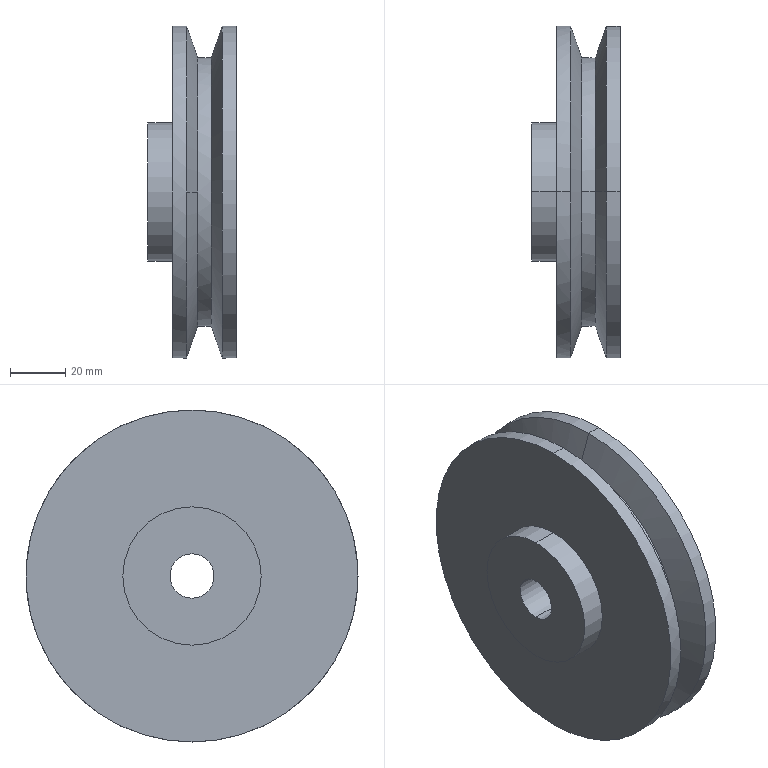Part | SolidWorks | features BaseBody 1 | 1 solid | 17 faces | box 32 x 120 x 120 mm | volume 235868 mm3 | cylinder 10 | cone 4 | plane 3 | commonest cylinder face diameters 120 x4 16 x2 50 x2 97.1 x2
STEP:
#1=CARTESIAN_POINT('',(-11.,0.,8.));
#2=VERTEX_POINT('',#1);
#3=CARTESIAN_POINT('',(-11.,0.,-8.));
#4=VERTEX_POINT('',#3);
#5=CARTESIAN_POINT('',(-11.,0.,0.));
#6=DIRECTION('',(1.,0.,0.));
#7=DIRECTION('',(0.,0.,-1.));
#8=AXIS2_PLACEMENT_3D('',#5,#6,#7);
#9=CIRCLE('',#8,8.);
#10=EDGE_CURVE('',#2,#4,#9,.T.);
#11=ORIENTED_EDGE('',*,*,#10,.F.);
#12=CARTESIAN_POINT('',(21.,0.,8.));
#13=VERTEX_POINT('',#12);
#14=CARTESIAN_POINT('',(0.,0.,8.));
#15=DIRECTION('',(1.,0.,0.));
#16=VECTOR('',#15,1000.);
#17=LINE('',#14,#16);
#18=EDGE_CURVE('',#2,#13,#17,.T.);
#19=ORIENTED_EDGE('',*,*,#18,.T.);
#20=CARTESIAN_POINT('',(21.,0.,-8.));
#21=VERTEX_POINT('',#20);
#22=CARTESIAN_POINT('',(21.,0.,0.));
#23=DIRECTION('',(-1.,0.,0.));
#24=DIRECTION('',(0.,0.,-1.));
#25=AXIS2_PLACEMENT_3D('',#22,#23,#24);
#26=CIRCLE('',#25,8.);
#27=EDGE_CURVE('',#21,#13,#26,.T.);
#28=ORIENTED_EDGE('',*,*,#27,.F.);
#29=CARTESIAN_POINT('',(0.,0.,-8.));
#30=DIRECTION('',(1.,0.,0.));
#31=VECTOR('',#30,1000.);
#32=LINE('',#29,#31);
#33=EDGE_CURVE('',#4,#21,#32,.T.);
#34=ORIENTED_EDGE('',*,*,#33,.F.);
#35=EDGE_LOOP('',(#11,#19,#28,#34));
#36=FACE_OUTER_BOUND('',#35,.T.);
#37=CARTESIAN_POINT('',(0.,0.,0.));
#38=DIRECTION('',(1.,0.,0.));
#39=DIRECTION('',(0.,0.,-1.));
#40=AXIS2_PLACEMENT_3D('',#37,#38,#39);
#41=CYLINDRICAL_SURFACE('',#40,8.);
#42=ADVANCED_FACE('',(#36),#41,.F.);
#43=CARTESIAN_POINT('',(15.947,0.,-60.));
#44=VERTEX_POINT('',#43);
#45=CARTESIAN_POINT('',(15.947,0.,60.));
#46=VERTEX_POINT('',#45);
#47=CARTESIAN_POINT('',(15.947,0.,0.));
#48=DIRECTION('',(1.,0.,0.));
#49=DIRECTION('',(0.,0.,-1.));
#50=AXIS2_PLACEMENT_3D('',#47,#48,#49);
#51=CIRCLE('',#50,60.);
#52=EDGE_CURVE('',#44,#46,#51,.T.);
#53=ORIENTED_EDGE('',*,*,#52,.T.);
#54=CARTESIAN_POINT('',(21.,0.,60.));
#55=VERTEX_POINT('',#54);
#56=CARTESIAN_POINT('',(0.,0.,60.));
#57=DIRECTION('',(1.,0.,0.));
#58=VECTOR('',#57,1000.);
#59=LINE('',#56,#58);
#60=EDGE_CURVE('',#46,#55,#59,.T.);
#61=ORIENTED_EDGE('',*,*,#60,.T.);
#62=CARTESIAN_POINT('',(21.,0.,-60.));
#63=VERTEX_POINT('',#62);
#64=CARTESIAN_POINT('',(21.,0.,0.));
#65=DIRECTION('',(1.,0.,0.));
#66=DIRECTION('',(0.,0.,-1.));
#67=AXIS2_PLACEMENT_3D('',#64,#65,#66);
#68=CIRCLE('',#67,60.);
#69=EDGE_CURVE('',#63,#55,#68,.T.);
#70=ORIENTED_EDGE('',*,*,#69,.F.);
#71=CARTESIAN_POINT('',(0.,0.,-60.));
#72=DIRECTION('',(1.,0.,0.));
#73=VECTOR('',#72,1000.);
#74=LINE('',#71,#73);
#75=EDGE_CURVE('',#44,#63,#74,.T.);
#76=ORIENTED_EDGE('',*,*,#75,.F.);
#77=EDGE_LOOP('',(#53,#61,#70,#76));
#78=FACE_OUTER_BOUND('',#77,.T.);
#79=CARTESIAN_POINT('',(0.,0.,0.));
#80=DIRECTION('',(1.,0.,0.));
#81=DIRECTION('',(0.,0.,-1.));
#82=AXIS2_PLACEMENT_3D('',#79,#80,#81);
#83=CYLINDRICAL_SURFACE('',#82,60.);
#84=ADVANCED_FACE('',(#78),#83,.T.);
#85=CARTESIAN_POINT('',(12.004,0.,-48.55));
#86=VERTEX_POINT('',#85);
#87=CARTESIAN_POINT('',(12.004,0.,48.55));
#88=VERTEX_POINT('',#87);
#89=CARTESIAN_POINT('',(12.004,0.,0.));
#90=DIRECTION('',(1.,0.,0.));
#91=DIRECTION('',(0.,0.,-1.));
#92=AXIS2_PLACEMENT_3D('',#89,#90,#91);
#93=CIRCLE('',#92,48.55);
#94=EDGE_CURVE('',#86,#88,#93,.T.);
#95=ORIENTED_EDGE('',*,*,#94,.T.);
#96=CARTESIAN_POINT('',(15.947,0.,60.));
#97=DIRECTION('',(0.3256,0.,0.9455));
#98=VECTOR('',#97,1000.);
#99=LINE('',#96,#98);
#100=EDGE_CURVE('',#88,#46,#99,.T.);
#101=ORIENTED_EDGE('',*,*,#100,.T.);
#102=ORIENTED_EDGE('',*,*,#52,.F.);
#103=CARTESIAN_POINT('',(15.947,0.,-60.));
#104=DIRECTION('',(0.3256,0.,-0.9455));
#105=VECTOR('',#104,1000.);
#106=LINE('',#103,#105);
#107=EDGE_CURVE('',#86,#44,#106,.T.);
#108=ORIENTED_EDGE('',*,*,#107,.F.);
#109=EDGE_LOOP('',(#95,#101,#102,#108));
#110=FACE_OUTER_BOUND('',#109,.T.);
#111=CARTESIAN_POINT('',(15.947,0.,0.));
#112=DIRECTION('',(1.,0.,0.));
#113=DIRECTION('',(0.,0.,-1.));
#114=AXIS2_PLACEMENT_3D('',#111,#112,#113);
#115=CONICAL_SURFACE('',#114,60.,1.239);
#116=ADVANCED_FACE('',(#110),#115,.T.);
#117=CARTESIAN_POINT('',(-11.,0.,25.));
#118=VERTEX_POINT('',#117);
#119=CARTESIAN_POINT('',(-11.,0.,-25.));
#120=VERTEX_POINT('',#119);
#121=CARTESIAN_POINT('',(-11.,0.,0.));
#122=DIRECTION('',(-1.,0.,0.));
#123=DIRECTION('',(0.,0.,-1.));
#124=AXIS2_PLACEMENT_3D('',#121,#122,#123);
#125=CIRCLE('',#124,25.);
#126=EDGE_CURVE('',#118,#120,#125,.T.);
#127=ORIENTED_EDGE('',*,*,#126,.F.);
#128=CARTESIAN_POINT('',(-2.,0.,25.));
#129=VERTEX_POINT('',#128);
#130=CARTESIAN_POINT('',(0.,0.,25.));
#131=DIRECTION('',(1.,0.,0.));
#132=VECTOR('',#131,1000.);
#133=LINE('',#130,#132);
#134=EDGE_CURVE('',#118,#129,#133,.T.);
#135=ORIENTED_EDGE('',*,*,#134,.T.);
#136=CARTESIAN_POINT('',(-2.,0.,-25.));
#137=VERTEX_POINT('',#136);
#138=CARTESIAN_POINT('',(-2.,0.,0.));
#139=DIRECTION('',(-1.,0.,0.));
#140=DIRECTION('',(0.,0.,-1.));
#141=AXIS2_PLACEMENT_3D('',#138,#139,#140);
#142=CIRCLE('',#141,25.);
#143=EDGE_CURVE('',#129,#137,#142,.T.);
#144=ORIENTED_EDGE('',*,*,#143,.T.);
#145=CARTESIAN_POINT('',(0.,0.,-25.));
#146=DIRECTION('',(1.,0.,0.));
#147=VECTOR('',#146,1000.);
#148=LINE('',#145,#147);
#149=EDGE_CURVE('',#120,#137,#148,.T.);
#150=ORIENTED_EDGE('',*,*,#149,.F.);
#151=EDGE_LOOP('',(#127,#135,#144,#150));
#152=FACE_OUTER_BOUND('',#151,.T.);
#153=CARTESIAN_POINT('',(0.,0.,0.));
#154=DIRECTION('',(1.,0.,0.));
#155=DIRECTION('',(0.,0.,-1.));
#156=AXIS2_PLACEMENT_3D('',#153,#154,#155);
#157=CYLINDRICAL_SURFACE('',#156,25.);
#158=ADVANCED_FACE('',(#152),#157,.T.);
#159=ORIENTED_EDGE('',*,*,#94,.F.);
#160=CARTESIAN_POINT('',(6.996,0.,-48.55));
#161=VERTEX_POINT('',#160);
#162=CARTESIAN_POINT('',(0.,0.,-48.55));
#163=DIRECTION('',(-1.,0.,0.));
#164=VECTOR('',#163,1000.);
#165=LINE('',#162,#164);
#166=EDGE_CURVE('',#86,#161,#165,.T.);
#167=ORIENTED_EDGE('',*,*,#166,.T.);
#168=CARTESIAN_POINT('',(6.996,48.55,0.));
#169=VERTEX_POINT('',#168);
#170=CARTESIAN_POINT('',(6.996,0.,0.));
#171=DIRECTION('',(1.,0.,0.));
#172=DIRECTION('',(0.,0.,1.));
#173=AXIS2_PLACEMENT_3D('',#170,#171,#172);
#174=CIRCLE('',#173,48.55);
#175=EDGE_CURVE('',#161,#169,#174,.T.);
#176=ORIENTED_EDGE('',*,*,#175,.T.);
#177=CARTESIAN_POINT('',(6.996,0.,48.55));
#178=VERTEX_POINT('',#177);
#179=CARTESIAN_POINT('',(6.996,0.,0.));
#180=DIRECTION('',(1.,0.,0.));
#181=DIRECTION('',(0.,0.,1.));
#182=AXIS2_PLACEMENT_3D('',#179,#180,#181);
#183=CIRCLE('',#182,48.55);
#184=EDGE_CURVE('',#169,#178,#183,.T.);
#185=ORIENTED_EDGE('',*,*,#184,.T.);
#186=CARTESIAN_POINT('',(0.,0.,48.55));
#187=DIRECTION('',(-1.,0.,0.));
#188=VECTOR('',#187,1000.);
#189=LINE('',#186,#188);
#190=EDGE_CURVE('',#88,#178,#189,.T.);
#191=ORIENTED_EDGE('',*,*,#190,.F.);
#192=EDGE_LOOP('',(#159,#167,#176,#185,#191));
#193=FACE_OUTER_BOUND('',#192,.T.);
#194=CARTESIAN_POINT('',(0.,0.,0.));
#195=DIRECTION('',(-1.,0.,0.));
#196=DIRECTION('',(0.,0.,1.));
#197=AXIS2_PLACEMENT_3D('',#194,#195,#196);
#198=CYLINDRICAL_SURFACE('',#197,48.55);
#199=ADVANCED_FACE('',(#193),#198,.T.);
#200=ORIENTED_EDGE('',*,*,#184,.F.);
#201=CARTESIAN_POINT('',(3.053,60.,0.));
#202=VERTEX_POINT('',#201);
#203=CARTESIAN_POINT('',(3.053,60.,0.));
#204=DIRECTION('',(-0.3256,0.9455,0.));
#205=VECTOR('',#204,1000.);
#206=LINE('',#203,#205);
#207=EDGE_CURVE('',#169,#202,#206,.T.);
#208=ORIENTED_EDGE('',*,*,#207,.T.);
#209=CARTESIAN_POINT('',(3.053,0.,60.));
#210=VERTEX_POINT('',#209);
#211=CARTESIAN_POINT('',(3.053,0.,0.));
#212=DIRECTION('',(1.,0.,0.));
#213=DIRECTION('',(0.,0.,1.));
#214=AXIS2_PLACEMENT_3D('',#211,#212,#213);
#215=CIRCLE('',#214,60.);
#216=EDGE_CURVE('',#202,#210,#215,.T.);
#217=ORIENTED_EDGE('',*,*,#216,.T.);
#218=CARTESIAN_POINT('',(3.053,-60.,0.));
#219=VERTEX_POINT('',#218);
#220=CARTESIAN_POINT('',(3.053,0.,0.));
#221=DIRECTION('',(1.,0.,0.));
#222=DIRECTION('',(0.,0.,1.));
#223=AXIS2_PLACEMENT_3D('',#220,#221,#222);
#224=CIRCLE('',#223,60.);
#225=EDGE_CURVE('',#210,#219,#224,.T.);
#226=ORIENTED_EDGE('',*,*,#225,.T.);
#227=CARTESIAN_POINT('',(6.996,-48.55,0.));
#228=VERTEX_POINT('',#227);
#229=CARTESIAN_POINT('',(3.053,-60.,0.));
#230=DIRECTION('',(-0.3256,-0.9455,0.));
#231=VECTOR('',#230,1000.);
#232=LINE('',#229,#231);
#233=EDGE_CURVE('',#228,#219,#232,.T.);
#234=ORIENTED_EDGE('',*,*,#233,.F.);
#235=CARTESIAN_POINT('',(6.996,0.,0.));
#236=DIRECTION('',(1.,0.,0.));
#237=DIRECTION('',(0.,0.,1.));
#238=AXIS2_PLACEMENT_3D('',#235,#236,#237);
#239=CIRCLE('',#238,48.55);
#240=EDGE_CURVE('',#178,#228,#239,.T.);
#241=ORIENTED_EDGE('',*,*,#240,.F.);
#242=EDGE_LOOP('',(#200,#208,#217,#226,#234,#241));
#243=FACE_OUTER_BOUND('',#242,.T.);
#244=CARTESIAN_POINT('',(3.053,0.,0.));
#245=DIRECTION('',(-1.,0.,0.));
#246=DIRECTION('',(0.,-1.,0.));
#247=AXIS2_PLACEMENT_3D('',#244,#245,#246);
#248=CONICAL_SURFACE('',#247,60.,1.239);
#249=ADVANCED_FACE('',(#243),#248,.T.);
#250=CARTESIAN_POINT('',(-2.,0.,60.));
#251=VERTEX_POINT('',#250);
#252=CARTESIAN_POINT('',(-2.,0.,-60.));
#253=VERTEX_POINT('',#252);
#254=CARTESIAN_POINT('',(-2.,0.,0.));
#255=DIRECTION('',(-1.,0.,0.));
#256=DIRECTION('',(0.,0.,-1.));
#257=AXIS2_PLACEMENT_3D('',#254,#255,#256);
#258=CIRCLE('',#257,60.);
#259=EDGE_CURVE('',#251,#253,#258,.T.);
#260=ORIENTED_EDGE('',*,*,#259,.F.);
#261=CARTESIAN_POINT('',(0.,0.,60.));
#262=DIRECTION('',(1.,0.,0.));
#263=VECTOR('',#262,1000.);
#264=LINE('',#261,#263);
#265=EDGE_CURVE('',#251,#210,#264,.T.);
#266=ORIENTED_EDGE('',*,*,#265,.T.);
#267=ORIENTED_EDGE('',*,*,#216,.F.);
#268=CARTESIAN_POINT('',(3.053,0.,-60.));
#269=VERTEX_POINT('',#268);
#270=CARTESIAN_POINT('',(3.053,0.,0.));
#271=DIRECTION('',(1.,0.,0.));
#272=DIRECTION('',(0.,0.,1.));
#273=AXIS2_PLACEMENT_3D('',#270,#271,#272);
#274=CIRCLE('',#273,60.);
#275=EDGE_CURVE('',#269,#202,#274,.T.);
#276=ORIENTED_EDGE('',*,*,#275,.F.);
#277=CARTESIAN_POINT('',(0.,0.,-60.));
#278=DIRECTION('',(1.,0.,0.));
#279=VECTOR('',#278,1000.);
#280=LINE('',#277,#279);
#281=EDGE_CURVE('',#253,#269,#280,.T.);
#282=ORIENTED_EDGE('',*,*,#281,.F.);
#283=EDGE_LOOP('',(#260,#266,#267,#276,#282));
#284=FACE_OUTER_BOUND('',#283,.T.);
#285=CARTESIAN_POINT('',(0.,0.,0.));
#286=DIRECTION('',(1.,0.,0.));
#287=DIRECTION('',(0.,0.,-1.));
#288=AXIS2_PLACEMENT_3D('',#285,#286,#287);
#289=CYLINDRICAL_SURFACE('',#288,60.);
#290=ADVANCED_FACE('',(#284),#289,.T.);
#291=ORIENTED_EDGE('',*,*,#27,.T.);
#292=CARTESIAN_POINT('',(21.,0.,0.));
#293=DIRECTION('',(-1.,0.,0.));
#294=DIRECTION('',(0.,0.,-1.));
#295=AXIS2_PLACEMENT_3D('',#292,#293,#294);
#296=CIRCLE('',#295,8.);
#297=EDGE_CURVE('',#13,#21,#296,.T.);
#298=ORIENTED_EDGE('',*,*,#297,.T.);
#299=EDGE_LOOP('',(#291,#298));
#300=FACE_BOUND('',#299,.T.);
#301=ORIENTED_EDGE('',*,*,#69,.T.);
#302=CARTESIAN_POINT('',(21.,0.,0.));
#303=DIRECTION('',(1.,0.,0.));
#304=DIRECTION('',(0.,0.,-1.));
#305=AXIS2_PLACEMENT_3D('',#302,#303,#304);
#306=CIRCLE('',#305,60.);
#307=EDGE_CURVE('',#55,#63,#306,.T.);
#308=ORIENTED_EDGE('',*,*,#307,.T.);
#309=EDGE_LOOP('',(#301,#308));
#310=FACE_OUTER_BOUND('',#309,.T.);
#311=CARTESIAN_POINT('',(21.,60.,0.));
#312=DIRECTION('',(1.,0.,0.));
#313=DIRECTION('',(0.,0.,-1.));
#314=AXIS2_PLACEMENT_3D('',#311,#312,#313);
#315=PLANE('',#314);
#316=ADVANCED_FACE('',(#300,#310),#315,.T.);
#317=ORIENTED_EDGE('',*,*,#18,.F.);
#318=CARTESIAN_POINT('',(-11.,0.,0.));
#319=DIRECTION('',(1.,0.,0.));
#320=DIRECTION('',(0.,0.,-1.));
#321=AXIS2_PLACEMENT_3D('',#318,#319,#320);
#322=CIRCLE('',#321,8.);
#323=EDGE_CURVE('',#4,#2,#322,.T.);
#324=ORIENTED_EDGE('',*,*,#323,.F.);
#325=ORIENTED_EDGE('',*,*,#33,.T.);
#326=ORIENTED_EDGE('',*,*,#297,.F.);
#327=EDGE_LOOP('',(#317,#324,#325,#326));
#328=FACE_OUTER_BOUND('',#327,.T.);
#329=CARTESIAN_POINT('',(0.,0.,0.));
#330=DIRECTION('',(1.,0.,0.));
#331=DIRECTION('',(0.,0.,-1.));
#332=AXIS2_PLACEMENT_3D('',#329,#330,#331);
#333=CYLINDRICAL_SURFACE('',#332,8.);
#334=ADVANCED_FACE('',(#328),#333,.F.);
#335=ORIENTED_EDGE('',*,*,#60,.F.);
#336=CARTESIAN_POINT('',(15.947,0.,0.));
#337=DIRECTION('',(1.,0.,0.));
#338=DIRECTION('',(0.,0.,-1.));
#339=AXIS2_PLACEMENT_3D('',#336,#337,#338);
#340=CIRCLE('',#339,60.);
#341=EDGE_CURVE('',#46,#44,#340,.T.);
#342=ORIENTED_EDGE('',*,*,#341,.T.);
#343=ORIENTED_EDGE('',*,*,#75,.T.);
#344=ORIENTED_EDGE('',*,*,#307,.F.);
#345=EDGE_LOOP('',(#335,#342,#343,#344));
#346=FACE_OUTER_BOUND('',#345,.T.);
#347=CARTESIAN_POINT('',(0.,0.,0.));
#348=DIRECTION('',(1.,0.,0.));
#349=DIRECTION('',(0.,0.,-1.));
#350=AXIS2_PLACEMENT_3D('',#347,#348,#349);
#351=CYLINDRICAL_SURFACE('',#350,60.);
#352=ADVANCED_FACE('',(#346),#351,.T.);
#353=CARTESIAN_POINT('',(-11.,0.,0.));
#354=DIRECTION('',(-1.,0.,0.));
#355=DIRECTION('',(0.,0.,-1.));
#356=AXIS2_PLACEMENT_3D('',#353,#354,#355);
#357=CIRCLE('',#356,25.);
#358=EDGE_CURVE('',#120,#118,#357,.T.);
#359=ORIENTED_EDGE('',*,*,#358,.T.);
#360=ORIENTED_EDGE('',*,*,#126,.T.);
#361=EDGE_LOOP('',(#359,#360));
#362=FACE_OUTER_BOUND('',#361,.T.);
#363=ORIENTED_EDGE('',*,*,#323,.T.);
#364=ORIENTED_EDGE('',*,*,#10,.T.);
#365=EDGE_LOOP('',(#363,#364));
#366=FACE_BOUND('',#365,.T.);
#367=CARTESIAN_POINT('',(-11.,0.,0.));
#368=DIRECTION('',(-1.,0.,0.));
#369=DIRECTION('',(0.,0.,1.));
#370=AXIS2_PLACEMENT_3D('',#367,#368,#369);
#371=PLANE('',#370);
#372=ADVANCED_FACE('',(#362,#366),#371,.T.);
#373=ORIENTED_EDGE('',*,*,#100,.F.);
#374=CARTESIAN_POINT('',(12.004,0.,0.));
#375=DIRECTION('',(1.,0.,0.));
#376=DIRECTION('',(0.,0.,-1.));
#377=AXIS2_PLACEMENT_3D('',#374,#375,#376);
#378=CIRCLE('',#377,48.55);
#379=EDGE_CURVE('',#88,#86,#378,.T.);
#380=ORIENTED_EDGE('',*,*,#379,.T.);
#381=ORIENTED_EDGE('',*,*,#107,.T.);
#382=ORIENTED_EDGE('',*,*,#341,.F.);
#383=EDGE_LOOP('',(#373,#380,#381,#382));
#384=FACE_OUTER_BOUND('',#383,.T.);
#385=CARTESIAN_POINT('',(15.947,0.,0.));
#386=DIRECTION('',(1.,0.,0.));
#387=DIRECTION('',(0.,0.,-1.));
#388=AXIS2_PLACEMENT_3D('',#385,#386,#387);
#389=CONICAL_SURFACE('',#388,60.,1.239);
#390=ADVANCED_FACE('',(#384),#389,.T.);
#391=ORIENTED_EDGE('',*,*,#134,.F.);
#392=ORIENTED_EDGE('',*,*,#358,.F.);
#393=ORIENTED_EDGE('',*,*,#149,.T.);
#394=CARTESIAN_POINT('',(-2.,0.,0.));
#395=DIRECTION('',(-1.,0.,0.));
#396=DIRECTION('',(0.,0.,-1.));
#397=AXIS2_PLACEMENT_3D('',#394,#395,#396);
#398=CIRCLE('',#397,25.);
#399=EDGE_CURVE('',#137,#129,#398,.T.);
#400=ORIENTED_EDGE('',*,*,#399,.T.);
#401=EDGE_LOOP('',(#391,#392,#393,#400));
#402=FACE_OUTER_BOUND('',#401,.T.);
#403=CARTESIAN_POINT('',(0.,0.,0.));
#404=DIRECTION('',(1.,0.,0.));
#405=DIRECTION('',(0.,0.,-1.));
#406=AXIS2_PLACEMENT_3D('',#403,#404,#405);
#407=CYLINDRICAL_SURFACE('',#406,25.);
#408=ADVANCED_FACE('',(#402),#407,.T.);
#409=ORIENTED_EDGE('',*,*,#166,.F.);
#410=ORIENTED_EDGE('',*,*,#379,.F.);
#411=ORIENTED_EDGE('',*,*,#190,.T.);
#412=ORIENTED_EDGE('',*,*,#240,.T.);
#413=CARTESIAN_POINT('',(6.996,0.,0.));
#414=DIRECTION('',(1.,0.,0.));
#415=DIRECTION('',(0.,0.,1.));
#416=AXIS2_PLACEMENT_3D('',#413,#414,#415);
#417=CIRCLE('',#416,48.55);
#418=EDGE_CURVE('',#228,#161,#417,.T.);
#419=ORIENTED_EDGE('',*,*,#418,.T.);
#420=EDGE_LOOP('',(#409,#410,#411,#412,#419));
#421=FACE_OUTER_BOUND('',#420,.T.);
#422=CARTESIAN_POINT('',(0.,0.,0.));
#423=DIRECTION('',(-1.,0.,0.));
#424=DIRECTION('',(0.,0.,1.));
#425=AXIS2_PLACEMENT_3D('',#422,#423,#424);
#426=CYLINDRICAL_SURFACE('',#425,48.55);
#427=ADVANCED_FACE('',(#421),#426,.T.);
#428=CARTESIAN_POINT('',(-2.,0.,0.));
#429=DIRECTION('',(-1.,0.,0.));
#430=DIRECTION('',(0.,0.,-1.));
#431=AXIS2_PLACEMENT_3D('',#428,#429,#430);
#432=CIRCLE('',#431,60.);
#433=EDGE_CURVE('',#253,#251,#432,.T.);
#434=ORIENTED_EDGE('',*,*,#433,.T.);
#435=ORIENTED_EDGE('',*,*,#259,.T.);
#436=EDGE_LOOP('',(#434,#435));
#437=FACE_OUTER_BOUND('',#436,.T.);
#438=ORIENTED_EDGE('',*,*,#399,.F.);
#439=ORIENTED_EDGE('',*,*,#143,.F.);
#440=EDGE_LOOP('',(#438,#439));
#441=FACE_BOUND('',#440,.T.);
#442=CARTESIAN_POINT('',(-2.,60.,0.));
#443=DIRECTION('',(-1.,0.,0.));
#444=DIRECTION('',(0.,0.,1.));
#445=AXIS2_PLACEMENT_3D('',#442,#443,#444);
#446=PLANE('',#445);
#447=ADVANCED_FACE('',(#437,#441),#446,.T.);
#448=ORIENTED_EDGE('',*,*,#207,.F.);
#449=ORIENTED_EDGE('',*,*,#175,.F.);
#450=ORIENTED_EDGE('',*,*,#418,.F.);
#451=ORIENTED_EDGE('',*,*,#233,.T.);
#452=CARTESIAN_POINT('',(3.053,0.,0.));
#453=DIRECTION('',(1.,0.,0.));
#454=DIRECTION('',(0.,0.,1.));
#455=AXIS2_PLACEMENT_3D('',#452,#453,#454);
#456=CIRCLE('',#455,60.);
#457=EDGE_CURVE('',#219,#269,#456,.T.);
#458=ORIENTED_EDGE('',*,*,#457,.T.);
#459=ORIENTED_EDGE('',*,*,#275,.T.);
#460=EDGE_LOOP('',(#448,#449,#450,#451,#458,#459));
#461=FACE_OUTER_BOUND('',#460,.T.);
#462=CARTESIAN_POINT('',(3.053,0.,0.));
#463=DIRECTION('',(-1.,0.,0.));
#464=DIRECTION('',(0.,-1.,0.));
#465=AXIS2_PLACEMENT_3D('',#462,#463,#464);
#466=CONICAL_SURFACE('',#465,60.,1.239);
#467=ADVANCED_FACE('',(#461),#466,.T.);
#468=ORIENTED_EDGE('',*,*,#265,.F.);
#469=ORIENTED_EDGE('',*,*,#433,.F.);
#470=ORIENTED_EDGE('',*,*,#281,.T.);
#471=ORIENTED_EDGE('',*,*,#457,.F.);
#472=ORIENTED_EDGE('',*,*,#225,.F.);
#473=EDGE_LOOP('',(#468,#469,#470,#471,#472));
#474=FACE_OUTER_BOUND('',#473,.T.);
#475=CARTESIAN_POINT('',(0.,0.,0.));
#476=DIRECTION('',(1.,0.,0.));
#477=DIRECTION('',(0.,0.,-1.));
#478=AXIS2_PLACEMENT_3D('',#475,#476,#477);
#479=CYLINDRICAL_SURFACE('',#478,60.);
#480=ADVANCED_FACE('',(#474),#479,.T.);
#481=CLOSED_SHELL('',(#42,#84,#116,#158,#199,#249,#290,#316,#334,#352,#372,#390,#408,#427,#447,#467,#480));
#482=MANIFOLD_SOLID_BREP('',#481);
#483=CARTESIAN_POINT('',(0.,0.,0.));
#484=DIRECTION('',(0.,0.,1.));
#485=DIRECTION('',(1.,0.,0.));
#486=AXIS2_PLACEMENT_3D('',#483,#484,#485);
#487=(LENGTH_UNIT()NAMED_UNIT(*)SI_UNIT(.MILLI.,.METRE.));
#488=UNCERTAINTY_MEASURE_WITH_UNIT(LENGTH_MEASURE(0.00001),#487,'','');
#489=(NAMED_UNIT(*)PLANE_ANGLE_UNIT()SI_UNIT($,.RADIAN.));
#490=(NAMED_UNIT(*)SI_UNIT($,.STERADIAN.)SOLID_ANGLE_UNIT());
#491=(GEOMETRIC_REPRESENTATION_CONTEXT(3)GLOBAL_UNCERTAINTY_ASSIGNED_CONTEXT((#488))GLOBAL_UNIT_ASSIGNED_CONTEXT((#487,#489,#490))REPRESENTATION_CONTEXT('',''));
#492=ADVANCED_BREP_SHAPE_REPRESENTATION('',(#482,#486),#491);